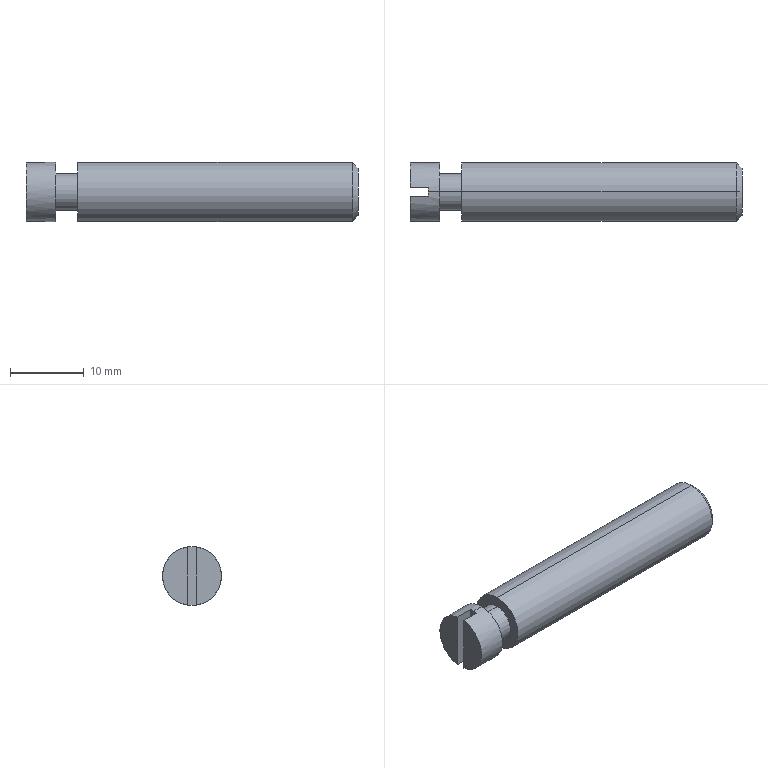Part | STEP file | 0217_Z_SBSPO8-45-1 | 1 solid | 16 faces | box 45 x 8 x 8 mm | volume 2139 mm3 | plane 8 | cylinder 6 | cone 2 | commonest cylinder face diameters 8 x4 5 x2
STEP:
#1=CARTESIAN_POINT('',(0.,0.,0.));
#2=DIRECTION('',(0.,0.,1.));
#3=DIRECTION('',(1.,0.,0.));
#4=AXIS2_PLACEMENT_3D('',#1,#2,#3);
#5=CARTESIAN_POINT('',(7.,0.,-4.));
#6=VERTEX_POINT('',#5);
#7=CARTESIAN_POINT('',(7.,0.,4.));
#8=VERTEX_POINT('',#7);
#9=CARTESIAN_POINT('',(7.,0.,0.));
#10=DIRECTION('',(1.,0.,0.));
#11=DIRECTION('',(0.,0.,-1.));
#12=AXIS2_PLACEMENT_3D('',#9,#10,#11);
#13=CIRCLE('',#12,4.);
#14=CARTESIAN_POINT('',(22.116,0.,0.));
#15=DIRECTION('',(1.,0.,0.));
#16=DIRECTION('',(0.,0.,-1.));
#17=AXIS2_PLACEMENT_3D('',#14,#15,#16);
#18=CYLINDRICAL_SURFACE('',#17,4.);
#19=CARTESIAN_POINT('',(0.,-15.117));
#20=DIRECTION('',(1.,0.));
#21=VECTOR('',#20,1.);
#22=LINE('',#19,#21);
#23=(GEOMETRIC_REPRESENTATION_CONTEXT(2)PARAMETRIC_REPRESENTATION_CONTEXT()REPRESENTATION_CONTEXT('',''));
#24=DEFINITIONAL_REPRESENTATION('',(#22),#23);
#25=PCURVE('',#18,#24);
#26=CARTESIAN_POINT('',(7.,4.,0.));
#27=DIRECTION('',(1.,0.,0.));
#28=DIRECTION('',(0.,0.,-1.));
#29=AXIS2_PLACEMENT_3D('',#26,#27,#28);
#30=PLANE('',#29);
#31=CARTESIAN_POINT('',(0.,-4.));
#32=DIRECTION('',(1.,0.));
#33=AXIS2_PLACEMENT_2D('',#31,#32);
#34=CIRCLE('',#33,4.);
#35=(GEOMETRIC_REPRESENTATION_CONTEXT(2)PARAMETRIC_REPRESENTATION_CONTEXT()REPRESENTATION_CONTEXT('',''));
#36=DEFINITIONAL_REPRESENTATION('',(#34),#35);
#37=PCURVE('',#30,#36);
#38=SURFACE_CURVE('',#13,(#25,#37),.PCURVE_S1.);
#39=EDGE_CURVE('',#6,#8,#38,.T.);
#40=ORIENTED_EDGE('',*,*,#39,.T.);
#41=CARTESIAN_POINT('',(44.233,0.,4.));
#42=VERTEX_POINT('',#41);
#43=CARTESIAN_POINT('',(22.116,0.,4.));
#44=DIRECTION('',(1.,0.,0.));
#45=VECTOR('',#44,1.);
#46=LINE('',#43,#45);
#47=CARTESIAN_POINT('',(3.142,0.));
#48=DIRECTION('',(0.,1.));
#49=VECTOR('',#48,1.);
#50=LINE('',#47,#49);
#51=(GEOMETRIC_REPRESENTATION_CONTEXT(2)PARAMETRIC_REPRESENTATION_CONTEXT()REPRESENTATION_CONTEXT('',''));
#52=DEFINITIONAL_REPRESENTATION('',(#50),#51);
#53=PCURVE('',#18,#52);
#54=CARTESIAN_POINT('',(22.116,0.,0.));
#55=DIRECTION('',(1.,0.,0.));
#56=DIRECTION('',(0.,0.,-1.));
#57=AXIS2_PLACEMENT_3D('',#54,#55,#56);
#58=CYLINDRICAL_SURFACE('',#57,4.);
#59=CARTESIAN_POINT('',(3.142,0.));
#60=DIRECTION('',(0.,1.));
#61=VECTOR('',#60,1.);
#62=LINE('',#59,#61);
#63=(GEOMETRIC_REPRESENTATION_CONTEXT(2)PARAMETRIC_REPRESENTATION_CONTEXT()REPRESENTATION_CONTEXT('',''));
#64=DEFINITIONAL_REPRESENTATION('',(#62),#63);
#65=PCURVE('',#58,#64);
#66=SURFACE_CURVE('',#46,(#53,#65),.PCURVE_S1.);
#67=EDGE_CURVE('',#8,#42,#66,.T.);
#68=ORIENTED_EDGE('',*,*,#67,.T.);
#69=CARTESIAN_POINT('',(44.233,0.,-4.));
#70=VERTEX_POINT('',#69);
#71=CARTESIAN_POINT('',(44.233,0.,0.));
#72=DIRECTION('',(-1.,0.,0.));
#73=DIRECTION('',(0.,0.,-1.));
#74=AXIS2_PLACEMENT_3D('',#71,#72,#73);
#75=CIRCLE('',#74,4.);
#76=CARTESIAN_POINT('',(6.283,22.116));
#77=DIRECTION('',(-1.,0.));
#78=VECTOR('',#77,1.);
#79=LINE('',#76,#78);
#80=(GEOMETRIC_REPRESENTATION_CONTEXT(2)PARAMETRIC_REPRESENTATION_CONTEXT()REPRESENTATION_CONTEXT('',''));
#81=DEFINITIONAL_REPRESENTATION('',(#79),#80);
#82=PCURVE('',#18,#81);
#83=CARTESIAN_POINT('',(44.233,0.,0.));
#84=DIRECTION('',(-1.,0.,0.));
#85=DIRECTION('',(0.,0.,1.));
#86=AXIS2_PLACEMENT_3D('',#83,#84,#85);
#87=CONICAL_SURFACE('',#86,4.,0.7854);
#88=CARTESIAN_POINT('',(-3.142,0.));
#89=DIRECTION('',(1.,0.));
#90=VECTOR('',#89,1.);
#91=LINE('',#88,#90);
#92=(GEOMETRIC_REPRESENTATION_CONTEXT(2)PARAMETRIC_REPRESENTATION_CONTEXT()REPRESENTATION_CONTEXT('',''));
#93=DEFINITIONAL_REPRESENTATION('',(#91),#92);
#94=PCURVE('',#87,#93);
#95=SURFACE_CURVE('',#75,(#82,#94),.PCURVE_S1.);
#96=EDGE_CURVE('',#42,#70,#95,.T.);
#97=ORIENTED_EDGE('',*,*,#96,.T.);
#98=CARTESIAN_POINT('',(22.116,0.,-4.));
#99=DIRECTION('',(1.,0.,0.));
#100=VECTOR('',#99,1.);
#101=LINE('',#98,#100);
#102=CARTESIAN_POINT('',(0.,0.));
#103=DIRECTION('',(0.,1.));
#104=VECTOR('',#103,1.);
#105=LINE('',#102,#104);
#106=(GEOMETRIC_REPRESENTATION_CONTEXT(2)PARAMETRIC_REPRESENTATION_CONTEXT()REPRESENTATION_CONTEXT('',''));
#107=DEFINITIONAL_REPRESENTATION('',(#105),#106);
#108=PCURVE('',#18,#107);
#109=CARTESIAN_POINT('',(6.283,0.));
#110=DIRECTION('',(0.,1.));
#111=VECTOR('',#110,1.);
#112=LINE('',#109,#111);
#113=(GEOMETRIC_REPRESENTATION_CONTEXT(2)PARAMETRIC_REPRESENTATION_CONTEXT()REPRESENTATION_CONTEXT('',''));
#114=DEFINITIONAL_REPRESENTATION('',(#112),#113);
#115=PCURVE('',#58,#114);
#116=SURFACE_CURVE('',#101,(#108,#115),.PCURVE_S1.);
#117=EDGE_CURVE('',#6,#70,#116,.T.);
#118=ORIENTED_EDGE('',*,*,#117,.F.);
#119=EDGE_LOOP('',(#40,#68,#97,#118));
#120=FACE_BOUND('',#119,.T.);
#121=ADVANCED_FACE('',(#120),#18,.T.);
#122=CARTESIAN_POINT('',(45.,0.,3.233));
#123=VERTEX_POINT('',#122);
#124=CARTESIAN_POINT('',(45.,0.,-3.233));
#125=VERTEX_POINT('',#124);
#126=CARTESIAN_POINT('',(45.,0.,0.));
#127=DIRECTION('',(-1.,0.,0.));
#128=DIRECTION('',(0.,0.,1.));
#129=AXIS2_PLACEMENT_3D('',#126,#127,#128);
#130=CIRCLE('',#129,3.233);
#131=CARTESIAN_POINT('',(0.,-0.767));
#132=DIRECTION('',(1.,0.));
#133=VECTOR('',#132,1.);
#134=LINE('',#131,#133);
#135=(GEOMETRIC_REPRESENTATION_CONTEXT(2)PARAMETRIC_REPRESENTATION_CONTEXT()REPRESENTATION_CONTEXT('',''));
#136=DEFINITIONAL_REPRESENTATION('',(#134),#135);
#137=PCURVE('',#87,#136);
#138=CARTESIAN_POINT('',(45.,1.617,0.));
#139=DIRECTION('',(1.,0.,0.));
#140=DIRECTION('',(0.,0.,-1.));
#141=AXIS2_PLACEMENT_3D('',#138,#139,#140);
#142=PLANE('',#141);
#143=CARTESIAN_POINT('',(-3.233,-1.617));
#144=CARTESIAN_POINT('',(-3.233,3.983));
#145=CARTESIAN_POINT('',(1.617,1.183));
#146=CARTESIAN_POINT('',(6.466,-1.617));
#147=CARTESIAN_POINT('',(1.617,-4.416));
#148=CARTESIAN_POINT('',(-3.233,-7.216));
#149=CARTESIAN_POINT('',(-3.233,-1.617));
#150=(BOUNDED_CURVE()B_SPLINE_CURVE(2,(#143,#144,#145,#146,#147,#148,#149),.UNSPECIFIED.,.T.,.F.)B_SPLINE_CURVE_WITH_KNOTS((1,2,2,2,2,1),(-2.094,0.,2.094,4.189,6.283,8.378),.UNSPECIFIED.)CURVE()GEOMETRIC_REPRESENTATION_ITEM()RATIONAL_B_SPLINE_CURVE((1.,0.5,1.,0.5,1.,0.5,1.))REPRESENTATION_ITEM(''));
#151=(GEOMETRIC_REPRESENTATION_CONTEXT(2)PARAMETRIC_REPRESENTATION_CONTEXT()REPRESENTATION_CONTEXT('',''));
#152=DEFINITIONAL_REPRESENTATION('',(#150),#151);
#153=PCURVE('',#142,#152);
#154=SURFACE_CURVE('',#130,(#137,#153),.PCURVE_S1.);
#155=EDGE_CURVE('',#123,#125,#154,.T.);
#156=ORIENTED_EDGE('',*,*,#155,.T.);
#157=CARTESIAN_POINT('',(44.233,0.,-4.));
#158=DIRECTION('',(-0.7071,0.,-0.7071));
#159=VECTOR('',#158,1.);
#160=LINE('',#157,#159);
#161=CARTESIAN_POINT('',(3.142,0.));
#162=DIRECTION('',(0.,1.));
#163=VECTOR('',#162,1.);
#164=LINE('',#161,#163);
#165=(GEOMETRIC_REPRESENTATION_CONTEXT(2)PARAMETRIC_REPRESENTATION_CONTEXT()REPRESENTATION_CONTEXT('',''));
#166=DEFINITIONAL_REPRESENTATION('',(#164),#165);
#167=PCURVE('',#87,#166);
#168=CARTESIAN_POINT('',(44.233,0.,0.));
#169=DIRECTION('',(-1.,0.,0.));
#170=DIRECTION('',(0.,0.,1.));
#171=AXIS2_PLACEMENT_3D('',#168,#169,#170);
#172=CONICAL_SURFACE('',#171,4.,0.7854);
#173=CARTESIAN_POINT('',(3.142,0.));
#174=DIRECTION('',(0.,1.));
#175=VECTOR('',#174,1.);
#176=LINE('',#173,#175);
#177=(GEOMETRIC_REPRESENTATION_CONTEXT(2)PARAMETRIC_REPRESENTATION_CONTEXT()REPRESENTATION_CONTEXT('',''));
#178=DEFINITIONAL_REPRESENTATION('',(#176),#177);
#179=PCURVE('',#172,#178);
#180=SURFACE_CURVE('',#160,(#167,#179),.PCURVE_S1.);
#181=EDGE_CURVE('',#125,#70,#180,.T.);
#182=ORIENTED_EDGE('',*,*,#181,.T.);
#183=ORIENTED_EDGE('',*,*,#96,.F.);
#184=CARTESIAN_POINT('',(44.233,0.,4.));
#185=DIRECTION('',(-0.7071,0.,0.7071));
#186=VECTOR('',#185,1.);
#187=LINE('',#184,#186);
#188=CARTESIAN_POINT('',(0.,0.));
#189=DIRECTION('',(0.,1.));
#190=VECTOR('',#189,1.);
#191=LINE('',#188,#190);
#192=(GEOMETRIC_REPRESENTATION_CONTEXT(2)PARAMETRIC_REPRESENTATION_CONTEXT()REPRESENTATION_CONTEXT('',''));
#193=DEFINITIONAL_REPRESENTATION('',(#191),#192);
#194=PCURVE('',#87,#193);
#195=CARTESIAN_POINT('',(6.283,0.));
#196=DIRECTION('',(0.,1.));
#197=VECTOR('',#196,1.);
#198=LINE('',#195,#197);
#199=(GEOMETRIC_REPRESENTATION_CONTEXT(2)PARAMETRIC_REPRESENTATION_CONTEXT()REPRESENTATION_CONTEXT('',''));
#200=DEFINITIONAL_REPRESENTATION('',(#198),#199);
#201=PCURVE('',#172,#200);
#202=SURFACE_CURVE('',#187,(#194,#201),.PCURVE_S1.);
#203=EDGE_CURVE('',#123,#42,#202,.T.);
#204=ORIENTED_EDGE('',*,*,#203,.F.);
#205=EDGE_LOOP('',(#156,#182,#183,#204));
#206=FACE_BOUND('',#205,.T.);
#207=ADVANCED_FACE('',(#206),#87,.T.);
#208=CARTESIAN_POINT('',(4.,0.,-2.5));
#209=VERTEX_POINT('',#208);
#210=CARTESIAN_POINT('',(4.,0.,2.5));
#211=VERTEX_POINT('',#210);
#212=CARTESIAN_POINT('',(4.,0.,0.));
#213=DIRECTION('',(1.,0.,0.));
#214=DIRECTION('',(0.,0.,-1.));
#215=AXIS2_PLACEMENT_3D('',#212,#213,#214);
#216=CIRCLE('',#215,2.5);
#217=CARTESIAN_POINT('',(5.5,0.,0.));
#218=DIRECTION('',(1.,0.,0.));
#219=DIRECTION('',(0.,0.,-1.));
#220=AXIS2_PLACEMENT_3D('',#217,#218,#219);
#221=CYLINDRICAL_SURFACE('',#220,2.5);
#222=CARTESIAN_POINT('',(0.,-1.5));
#223=DIRECTION('',(1.,0.));
#224=VECTOR('',#223,1.);
#225=LINE('',#222,#224);
#226=(GEOMETRIC_REPRESENTATION_CONTEXT(2)PARAMETRIC_REPRESENTATION_CONTEXT()REPRESENTATION_CONTEXT('',''));
#227=DEFINITIONAL_REPRESENTATION('',(#225),#226);
#228=PCURVE('',#221,#227);
#229=CARTESIAN_POINT('',(4.,4.,0.));
#230=DIRECTION('',(-1.,0.,0.));
#231=DIRECTION('',(0.,0.,1.));
#232=AXIS2_PLACEMENT_3D('',#229,#230,#231);
#233=PLANE('',#232);
#234=CARTESIAN_POINT('',(-2.5,-4.));
#235=CARTESIAN_POINT('',(-2.5,0.3301));
#236=CARTESIAN_POINT('',(1.25,-1.835));
#237=CARTESIAN_POINT('',(5.,-4.));
#238=CARTESIAN_POINT('',(1.25,-6.165));
#239=CARTESIAN_POINT('',(-2.5,-8.33));
#240=CARTESIAN_POINT('',(-2.5,-4.));
#241=(BOUNDED_CURVE()B_SPLINE_CURVE(2,(#234,#235,#236,#237,#238,#239,#240),.UNSPECIFIED.,.T.,.F.)B_SPLINE_CURVE_WITH_KNOTS((1,2,2,2,2,1),(-2.094,0.,2.094,4.189,6.283,8.378),.UNSPECIFIED.)CURVE()GEOMETRIC_REPRESENTATION_ITEM()RATIONAL_B_SPLINE_CURVE((1.,0.5,1.,0.5,1.,0.5,1.))REPRESENTATION_ITEM(''));
#242=(GEOMETRIC_REPRESENTATION_CONTEXT(2)PARAMETRIC_REPRESENTATION_CONTEXT()REPRESENTATION_CONTEXT('',''));
#243=DEFINITIONAL_REPRESENTATION('',(#241),#242);
#244=PCURVE('',#233,#243);
#245=SURFACE_CURVE('',#216,(#228,#244),.PCURVE_S1.);
#246=EDGE_CURVE('',#209,#211,#245,.T.);
#247=ORIENTED_EDGE('',*,*,#246,.T.);
#248=CARTESIAN_POINT('',(7.,0.,2.5));
#249=VERTEX_POINT('',#248);
#250=CARTESIAN_POINT('',(5.5,0.,2.5));
#251=DIRECTION('',(1.,0.,0.));
#252=VECTOR('',#251,1.);
#253=LINE('',#250,#252);
#254=CARTESIAN_POINT('',(3.142,0.));
#255=DIRECTION('',(0.,1.));
#256=VECTOR('',#255,1.);
#257=LINE('',#254,#256);
#258=(GEOMETRIC_REPRESENTATION_CONTEXT(2)PARAMETRIC_REPRESENTATION_CONTEXT()REPRESENTATION_CONTEXT('',''));
#259=DEFINITIONAL_REPRESENTATION('',(#257),#258);
#260=PCURVE('',#221,#259);
#261=CARTESIAN_POINT('',(5.5,0.,0.));
#262=DIRECTION('',(1.,0.,0.));
#263=DIRECTION('',(0.,0.,-1.));
#264=AXIS2_PLACEMENT_3D('',#261,#262,#263);
#265=CYLINDRICAL_SURFACE('',#264,2.5);
#266=CARTESIAN_POINT('',(3.142,0.));
#267=DIRECTION('',(0.,1.));
#268=VECTOR('',#267,1.);
#269=LINE('',#266,#268);
#270=(GEOMETRIC_REPRESENTATION_CONTEXT(2)PARAMETRIC_REPRESENTATION_CONTEXT()REPRESENTATION_CONTEXT('',''));
#271=DEFINITIONAL_REPRESENTATION('',(#269),#270);
#272=PCURVE('',#265,#271);
#273=SURFACE_CURVE('',#253,(#260,#272),.PCURVE_S1.);
#274=EDGE_CURVE('',#211,#249,#273,.T.);
#275=ORIENTED_EDGE('',*,*,#274,.T.);
#276=CARTESIAN_POINT('',(7.,0.,-2.5));
#277=VERTEX_POINT('',#276);
#278=CARTESIAN_POINT('',(7.,0.,0.));
#279=DIRECTION('',(-1.,0.,0.));
#280=DIRECTION('',(0.,0.,-1.));
#281=AXIS2_PLACEMENT_3D('',#278,#279,#280);
#282=CIRCLE('',#281,2.5);
#283=CARTESIAN_POINT('',(6.283,1.5));
#284=DIRECTION('',(-1.,0.));
#285=VECTOR('',#284,1.);
#286=LINE('',#283,#285);
#287=(GEOMETRIC_REPRESENTATION_CONTEXT(2)PARAMETRIC_REPRESENTATION_CONTEXT()REPRESENTATION_CONTEXT('',''));
#288=DEFINITIONAL_REPRESENTATION('',(#286),#287);
#289=PCURVE('',#221,#288);
#290=CARTESIAN_POINT('',(2.5,-4.));
#291=CARTESIAN_POINT('',(2.5,-8.33));
#292=CARTESIAN_POINT('',(-1.25,-6.165));
#293=CARTESIAN_POINT('',(-5.,-4.));
#294=CARTESIAN_POINT('',(-1.25,-1.835));
#295=CARTESIAN_POINT('',(2.5,0.3301));
#296=CARTESIAN_POINT('',(2.5,-4.));
#297=(BOUNDED_CURVE()B_SPLINE_CURVE(2,(#290,#291,#292,#293,#294,#295,#296),.UNSPECIFIED.,.T.,.F.)B_SPLINE_CURVE_WITH_KNOTS((1,2,2,2,2,1),(-2.094,0.,2.094,4.189,6.283,8.378),.UNSPECIFIED.)CURVE()GEOMETRIC_REPRESENTATION_ITEM()RATIONAL_B_SPLINE_CURVE((1.,0.5,1.,0.5,1.,0.5,1.))REPRESENTATION_ITEM(''));
#298=(GEOMETRIC_REPRESENTATION_CONTEXT(2)PARAMETRIC_REPRESENTATION_CONTEXT()REPRESENTATION_CONTEXT('',''));
#299=DEFINITIONAL_REPRESENTATION('',(#297),#298);
#300=PCURVE('',#30,#299);
#301=SURFACE_CURVE('',#282,(#289,#300),.PCURVE_S1.);
#302=EDGE_CURVE('',#249,#277,#301,.T.);
#303=ORIENTED_EDGE('',*,*,#302,.T.);
#304=CARTESIAN_POINT('',(5.5,0.,-2.5));
#305=DIRECTION('',(1.,0.,0.));
#306=VECTOR('',#305,1.);
#307=LINE('',#304,#306);
#308=CARTESIAN_POINT('',(0.,0.));
#309=DIRECTION('',(0.,1.));
#310=VECTOR('',#309,1.);
#311=LINE('',#308,#310);
#312=(GEOMETRIC_REPRESENTATION_CONTEXT(2)PARAMETRIC_REPRESENTATION_CONTEXT()REPRESENTATION_CONTEXT('',''));
#313=DEFINITIONAL_REPRESENTATION('',(#311),#312);
#314=PCURVE('',#221,#313);
#315=CARTESIAN_POINT('',(6.283,0.));
#316=DIRECTION('',(0.,1.));
#317=VECTOR('',#316,1.);
#318=LINE('',#315,#317);
#319=(GEOMETRIC_REPRESENTATION_CONTEXT(2)PARAMETRIC_REPRESENTATION_CONTEXT()REPRESENTATION_CONTEXT('',''));
#320=DEFINITIONAL_REPRESENTATION('',(#318),#319);
#321=PCURVE('',#265,#320);
#322=SURFACE_CURVE('',#307,(#314,#321),.PCURVE_S1.);
#323=EDGE_CURVE('',#209,#277,#322,.T.);
#324=ORIENTED_EDGE('',*,*,#323,.F.);
#325=EDGE_LOOP('',(#247,#275,#303,#324));
#326=FACE_BOUND('',#325,.T.);
#327=ADVANCED_FACE('',(#326),#221,.T.);
#328=CARTESIAN_POINT('',(2.5,0.6,3.955));
#329=VERTEX_POINT('',#328);
#330=CARTESIAN_POINT('',(2.5,0.,4.));
#331=VERTEX_POINT('',#330);
#332=CARTESIAN_POINT('',(2.5,0.,0.));
#333=DIRECTION('',(1.,0.,0.));
#334=DIRECTION('',(0.,0.,-1.));
#335=AXIS2_PLACEMENT_3D('',#332,#333,#334);
#336=CIRCLE('',#335,4.);
#337=CARTESIAN_POINT('',(22.116,0.,0.));
#338=DIRECTION('',(1.,0.,0.));
#339=DIRECTION('',(0.,0.,-1.));
#340=AXIS2_PLACEMENT_3D('',#337,#338,#339);
#341=CYLINDRICAL_SURFACE('',#340,4.);
#342=CARTESIAN_POINT('',(0.,-19.616));
#343=DIRECTION('',(1.,0.));
#344=VECTOR('',#343,1.);
#345=LINE('',#342,#344);
#346=(GEOMETRIC_REPRESENTATION_CONTEXT(2)PARAMETRIC_REPRESENTATION_CONTEXT()REPRESENTATION_CONTEXT('',''));
#347=DEFINITIONAL_REPRESENTATION('',(#345),#346);
#348=PCURVE('',#341,#347);
#349=CARTESIAN_POINT('',(2.5,-0.6,4.));
#350=DIRECTION('',(1.,0.,0.));
#351=DIRECTION('',(0.,0.,-1.));
#352=AXIS2_PLACEMENT_3D('',#349,#350,#351);
#353=PLANE('',#352);
#354=CARTESIAN_POINT('',(4.,0.6));
#355=DIRECTION('',(1.,0.));
#356=AXIS2_PLACEMENT_2D('',#354,#355);
#357=CIRCLE('',#356,4.);
#358=(GEOMETRIC_REPRESENTATION_CONTEXT(2)PARAMETRIC_REPRESENTATION_CONTEXT()REPRESENTATION_CONTEXT('',''));
#359=DEFINITIONAL_REPRESENTATION('',(#357),#358);
#360=PCURVE('',#353,#359);
#361=SURFACE_CURVE('',#336,(#348,#360),.PCURVE_S1.);
#362=EDGE_CURVE('',#329,#331,#361,.T.);
#363=ORIENTED_EDGE('',*,*,#362,.T.);
#364=CARTESIAN_POINT('',(4.,0.,4.));
#365=VERTEX_POINT('',#364);
#366=CARTESIAN_POINT('',(22.116,0.,4.));
#367=DIRECTION('',(1.,0.,0.));
#368=VECTOR('',#367,1.);
#369=LINE('',#366,#368);
#370=CARTESIAN_POINT('',(3.142,0.));
#371=DIRECTION('',(0.,1.));
#372=VECTOR('',#371,1.);
#373=LINE('',#370,#372);
#374=(GEOMETRIC_REPRESENTATION_CONTEXT(2)PARAMETRIC_REPRESENTATION_CONTEXT()REPRESENTATION_CONTEXT('',''));
#375=DEFINITIONAL_REPRESENTATION('',(#373),#374);
#376=PCURVE('',#341,#375);
#377=CARTESIAN_POINT('',(22.116,0.,0.));
#378=DIRECTION('',(1.,0.,0.));
#379=DIRECTION('',(0.,0.,-1.));
#380=AXIS2_PLACEMENT_3D('',#377,#378,#379);
#381=CYLINDRICAL_SURFACE('',#380,4.);
#382=CARTESIAN_POINT('',(3.142,0.));
#383=DIRECTION('',(0.,1.));
#384=VECTOR('',#383,1.);
#385=LINE('',#382,#384);
#386=(GEOMETRIC_REPRESENTATION_CONTEXT(2)PARAMETRIC_REPRESENTATION_CONTEXT()REPRESENTATION_CONTEXT('',''));
#387=DEFINITIONAL_REPRESENTATION('',(#385),#386);
#388=PCURVE('',#381,#387);
#389=SURFACE_CURVE('',#369,(#376,#388),.PCURVE_S1.);
#390=EDGE_CURVE('',#331,#365,#389,.T.);
#391=ORIENTED_EDGE('',*,*,#390,.T.);
#392=CARTESIAN_POINT('',(4.,0.,-4.));
#393=VERTEX_POINT('',#392);
#394=CARTESIAN_POINT('',(4.,0.,0.));
#395=DIRECTION('',(-1.,0.,0.));
#396=DIRECTION('',(0.,0.,-1.));
#397=AXIS2_PLACEMENT_3D('',#394,#395,#396);
#398=CIRCLE('',#397,4.);
#399=CARTESIAN_POINT('',(6.283,-18.116));
#400=DIRECTION('',(-1.,0.));
#401=VECTOR('',#400,1.);
#402=LINE('',#399,#401);
#403=(GEOMETRIC_REPRESENTATION_CONTEXT(2)PARAMETRIC_REPRESENTATION_CONTEXT()REPRESENTATION_CONTEXT('',''));
#404=DEFINITIONAL_REPRESENTATION('',(#402),#403);
#405=PCURVE('',#341,#404);
#406=CARTESIAN_POINT('',(0.,-4.));
#407=DIRECTION('',(-1.,0.));
#408=AXIS2_PLACEMENT_2D('',#406,#407);
#409=CIRCLE('',#408,4.);
#410=(GEOMETRIC_REPRESENTATION_CONTEXT(2)PARAMETRIC_REPRESENTATION_CONTEXT()REPRESENTATION_CONTEXT('',''));
#411=DEFINITIONAL_REPRESENTATION('',(#409),#410);
#412=PCURVE('',#233,#411);
#413=SURFACE_CURVE('',#398,(#405,#412),.PCURVE_S1.);
#414=EDGE_CURVE('',#365,#393,#413,.T.);
#415=ORIENTED_EDGE('',*,*,#414,.T.);
#416=CARTESIAN_POINT('',(2.5,0.,-4.));
#417=VERTEX_POINT('',#416);
#418=CARTESIAN_POINT('',(22.116,0.,-4.));
#419=DIRECTION('',(1.,0.,0.));
#420=VECTOR('',#419,1.);
#421=LINE('',#418,#420);
#422=CARTESIAN_POINT('',(0.,0.));
#423=DIRECTION('',(0.,1.));
#424=VECTOR('',#423,1.);
#425=LINE('',#422,#424);
#426=(GEOMETRIC_REPRESENTATION_CONTEXT(2)PARAMETRIC_REPRESENTATION_CONTEXT()REPRESENTATION_CONTEXT('',''));
#427=DEFINITIONAL_REPRESENTATION('',(#425),#426);
#428=PCURVE('',#341,#427);
#429=CARTESIAN_POINT('',(6.283,0.));
#430=DIRECTION('',(0.,1.));
#431=VECTOR('',#430,1.);
#432=LINE('',#429,#431);
#433=(GEOMETRIC_REPRESENTATION_CONTEXT(2)PARAMETRIC_REPRESENTATION_CONTEXT()REPRESENTATION_CONTEXT('',''));
#434=DEFINITIONAL_REPRESENTATION('',(#432),#433);
#435=PCURVE('',#381,#434);
#436=SURFACE_CURVE('',#421,(#428,#435),.PCURVE_S1.);
#437=EDGE_CURVE('',#417,#393,#436,.T.);
#438=ORIENTED_EDGE('',*,*,#437,.F.);
#439=CARTESIAN_POINT('',(2.5,0.6,-3.955));
#440=VERTEX_POINT('',#439);
#441=CARTESIAN_POINT('',(2.5,0.,0.));
#442=DIRECTION('',(1.,0.,0.));
#443=DIRECTION('',(0.,0.,-1.));
#444=AXIS2_PLACEMENT_3D('',#441,#442,#443);
#445=CIRCLE('',#444,4.);
#446=CARTESIAN_POINT('',(0.,-19.616));
#447=DIRECTION('',(1.,0.));
#448=VECTOR('',#447,1.);
#449=LINE('',#446,#448);
#450=(GEOMETRIC_REPRESENTATION_CONTEXT(2)PARAMETRIC_REPRESENTATION_CONTEXT()REPRESENTATION_CONTEXT('',''));
#451=DEFINITIONAL_REPRESENTATION('',(#449),#450);
#452=PCURVE('',#341,#451);
#453=CARTESIAN_POINT('',(4.,0.6));
#454=DIRECTION('',(1.,0.));
#455=AXIS2_PLACEMENT_2D('',#453,#454);
#456=CIRCLE('',#455,4.);
#457=(GEOMETRIC_REPRESENTATION_CONTEXT(2)PARAMETRIC_REPRESENTATION_CONTEXT()REPRESENTATION_CONTEXT('',''));
#458=DEFINITIONAL_REPRESENTATION('',(#456),#457);
#459=PCURVE('',#353,#458);
#460=SURFACE_CURVE('',#445,(#452,#459),.PCURVE_S1.);
#461=EDGE_CURVE('',#417,#440,#460,.T.);
#462=ORIENTED_EDGE('',*,*,#461,.T.);
#463=CARTESIAN_POINT('',(0.,0.6,-3.955));
#464=VERTEX_POINT('',#463);
#465=CARTESIAN_POINT('',(22.116,0.6,-3.955));
#466=DIRECTION('',(-1.,0.,0.));
#467=VECTOR('',#466,1.);
#468=LINE('',#465,#467);
#469=CARTESIAN_POINT('',(0.1506,0.));
#470=DIRECTION('',(0.,-1.));
#471=VECTOR('',#470,1.);
#472=LINE('',#469,#471);
#473=(GEOMETRIC_REPRESENTATION_CONTEXT(2)PARAMETRIC_REPRESENTATION_CONTEXT()REPRESENTATION_CONTEXT('',''));
#474=DEFINITIONAL_REPRESENTATION('',(#472),#473);
#475=PCURVE('',#341,#474);
#476=CARTESIAN_POINT('',(2.5,0.6,4.));
#477=DIRECTION('',(0.,1.,0.));
#478=DIRECTION('',(0.,0.,1.));
#479=AXIS2_PLACEMENT_3D('',#476,#477,#478);
#480=PLANE('',#479);
#481=CARTESIAN_POINT('',(-7.955,19.616));
#482=DIRECTION('',(0.,-1.));
#483=VECTOR('',#482,1.);
#484=LINE('',#481,#483);
#485=(GEOMETRIC_REPRESENTATION_CONTEXT(2)PARAMETRIC_REPRESENTATION_CONTEXT()REPRESENTATION_CONTEXT('',''));
#486=DEFINITIONAL_REPRESENTATION('',(#484),#485);
#487=PCURVE('',#480,#486);
#488=SURFACE_CURVE('',#468,(#475,#487),.PCURVE_S1.);
#489=EDGE_CURVE('',#440,#464,#488,.T.);
#490=ORIENTED_EDGE('',*,*,#489,.T.);
#491=CARTESIAN_POINT('',(0.,0.6,3.955));
#492=VERTEX_POINT('',#491);
#493=CARTESIAN_POINT('',(0.,0.,0.));
#494=DIRECTION('',(1.,0.,0.));
#495=DIRECTION('',(0.,0.,-1.));
#496=AXIS2_PLACEMENT_3D('',#493,#494,#495);
#497=CIRCLE('',#496,4.);
#498=CARTESIAN_POINT('',(0.,-22.116));
#499=DIRECTION('',(1.,0.));
#500=VECTOR('',#499,1.);
#501=LINE('',#498,#500);
#502=(GEOMETRIC_REPRESENTATION_CONTEXT(2)PARAMETRIC_REPRESENTATION_CONTEXT()REPRESENTATION_CONTEXT('',''));
#503=DEFINITIONAL_REPRESENTATION('',(#501),#502);
#504=PCURVE('',#341,#503);
#505=CARTESIAN_POINT('',(0.,2.,0.));
#506=DIRECTION('',(-1.,0.,0.));
#507=DIRECTION('',(0.,0.,1.));
#508=AXIS2_PLACEMENT_3D('',#505,#506,#507);
#509=PLANE('',#508);
#510=CARTESIAN_POINT('',(-4.,-2.));
#511=CARTESIAN_POINT('',(-4.,4.928));
#512=CARTESIAN_POINT('',(2.,1.464));
#513=CARTESIAN_POINT('',(8.,-2.));
#514=CARTESIAN_POINT('',(2.,-5.464));
#515=CARTESIAN_POINT('',(-4.,-8.928));
#516=CARTESIAN_POINT('',(-4.,-2.));
#517=(BOUNDED_CURVE()B_SPLINE_CURVE(2,(#510,#511,#512,#513,#514,#515,#516),.UNSPECIFIED.,.T.,.F.)B_SPLINE_CURVE_WITH_KNOTS((1,2,2,2,2,1),(-2.094,0.,2.094,4.189,6.283,8.378),.UNSPECIFIED.)CURVE()GEOMETRIC_REPRESENTATION_ITEM()RATIONAL_B_SPLINE_CURVE((1.,0.5,1.,0.5,1.,0.5,1.))REPRESENTATION_ITEM(''));
#518=(GEOMETRIC_REPRESENTATION_CONTEXT(2)PARAMETRIC_REPRESENTATION_CONTEXT()REPRESENTATION_CONTEXT('',''));
#519=DEFINITIONAL_REPRESENTATION('',(#517),#518);
#520=PCURVE('',#509,#519);
#521=SURFACE_CURVE('',#497,(#504,#520),.PCURVE_S1.);
#522=EDGE_CURVE('',#464,#492,#521,.T.);
#523=ORIENTED_EDGE('',*,*,#522,.T.);
#524=CARTESIAN_POINT('',(22.116,0.6,3.955));
#525=DIRECTION('',(1.,0.,0.));
#526=VECTOR('',#525,1.);
#527=LINE('',#524,#526);
#528=CARTESIAN_POINT('',(2.991,0.));
#529=DIRECTION('',(0.,1.));
#530=VECTOR('',#529,1.);
#531=LINE('',#528,#530);
#532=(GEOMETRIC_REPRESENTATION_CONTEXT(2)PARAMETRIC_REPRESENTATION_CONTEXT()REPRESENTATION_CONTEXT('',''));
#533=DEFINITIONAL_REPRESENTATION('',(#531),#532);
#534=PCURVE('',#341,#533);
#535=CARTESIAN_POINT('',(-0.04526,19.616));
#536=DIRECTION('',(0.,1.));
#537=VECTOR('',#536,1.);
#538=LINE('',#535,#537);
#539=(GEOMETRIC_REPRESENTATION_CONTEXT(2)PARAMETRIC_REPRESENTATION_CONTEXT()REPRESENTATION_CONTEXT('',''));
#540=DEFINITIONAL_REPRESENTATION('',(#538),#539);
#541=PCURVE('',#480,#540);
#542=SURFACE_CURVE('',#527,(#534,#541),.PCURVE_S1.);
#543=EDGE_CURVE('',#492,#329,#542,.T.);
#544=ORIENTED_EDGE('',*,*,#543,.T.);
#545=EDGE_LOOP('',(#363,#391,#415,#438,#462,#490,#523,#544));
#546=FACE_BOUND('',#545,.T.);
#547=ADVANCED_FACE('',(#546),#341,.T.);
#548=ORIENTED_EDGE('',*,*,#67,.F.);
#549=CARTESIAN_POINT('',(7.,0.,0.));
#550=DIRECTION('',(1.,0.,0.));
#551=DIRECTION('',(0.,0.,-1.));
#552=AXIS2_PLACEMENT_3D('',#549,#550,#551);
#553=CIRCLE('',#552,4.);
#554=CARTESIAN_POINT('',(0.,-15.117));
#555=DIRECTION('',(1.,0.));
#556=VECTOR('',#555,1.);
#557=LINE('',#554,#556);
#558=(GEOMETRIC_REPRESENTATION_CONTEXT(2)PARAMETRIC_REPRESENTATION_CONTEXT()REPRESENTATION_CONTEXT('',''));
#559=DEFINITIONAL_REPRESENTATION('',(#557),#558);
#560=PCURVE('',#58,#559);
#561=CARTESIAN_POINT('',(0.,-4.));
#562=DIRECTION('',(1.,0.));
#563=AXIS2_PLACEMENT_2D('',#561,#562);
#564=CIRCLE('',#563,4.);
#565=(GEOMETRIC_REPRESENTATION_CONTEXT(2)PARAMETRIC_REPRESENTATION_CONTEXT()REPRESENTATION_CONTEXT('',''));
#566=DEFINITIONAL_REPRESENTATION('',(#564),#565);
#567=PCURVE('',#30,#566);
#568=SURFACE_CURVE('',#553,(#560,#567),.PCURVE_S1.);
#569=EDGE_CURVE('',#8,#6,#568,.T.);
#570=ORIENTED_EDGE('',*,*,#569,.T.);
#571=ORIENTED_EDGE('',*,*,#117,.T.);
#572=CARTESIAN_POINT('',(44.233,0.,0.));
#573=DIRECTION('',(-1.,0.,0.));
#574=DIRECTION('',(0.,0.,-1.));
#575=AXIS2_PLACEMENT_3D('',#572,#573,#574);
#576=CIRCLE('',#575,4.);
#577=CARTESIAN_POINT('',(6.283,22.116));
#578=DIRECTION('',(-1.,0.));
#579=VECTOR('',#578,1.);
#580=LINE('',#577,#579);
#581=(GEOMETRIC_REPRESENTATION_CONTEXT(2)PARAMETRIC_REPRESENTATION_CONTEXT()REPRESENTATION_CONTEXT('',''));
#582=DEFINITIONAL_REPRESENTATION('',(#580),#581);
#583=PCURVE('',#58,#582);
#584=CARTESIAN_POINT('',(3.142,0.));
#585=DIRECTION('',(1.,0.));
#586=VECTOR('',#585,1.);
#587=LINE('',#584,#586);
#588=(GEOMETRIC_REPRESENTATION_CONTEXT(2)PARAMETRIC_REPRESENTATION_CONTEXT()REPRESENTATION_CONTEXT('',''));
#589=DEFINITIONAL_REPRESENTATION('',(#587),#588);
#590=PCURVE('',#172,#589);
#591=SURFACE_CURVE('',#576,(#583,#590),.PCURVE_S1.);
#592=EDGE_CURVE('',#70,#42,#591,.T.);
#593=ORIENTED_EDGE('',*,*,#592,.T.);
#594=EDGE_LOOP('',(#548,#570,#571,#593));
#595=FACE_BOUND('',#594,.T.);
#596=ADVANCED_FACE('',(#595),#58,.T.);
#597=CARTESIAN_POINT('',(7.,0.,0.));
#598=DIRECTION('',(-1.,0.,0.));
#599=DIRECTION('',(0.,0.,-1.));
#600=AXIS2_PLACEMENT_3D('',#597,#598,#599);
#601=CIRCLE('',#600,2.5);
#602=CARTESIAN_POINT('',(2.5,-4.));
#603=CARTESIAN_POINT('',(2.5,-8.33));
#604=CARTESIAN_POINT('',(-1.25,-6.165));
#605=CARTESIAN_POINT('',(-5.,-4.));
#606=CARTESIAN_POINT('',(-1.25,-1.835));
#607=CARTESIAN_POINT('',(2.5,0.3301));
#608=CARTESIAN_POINT('',(2.5,-4.));
#609=(BOUNDED_CURVE()B_SPLINE_CURVE(2,(#602,#603,#604,#605,#606,#607,#608),.UNSPECIFIED.,.T.,.F.)B_SPLINE_CURVE_WITH_KNOTS((1,2,2,2,2,1),(-2.094,0.,2.094,4.189,6.283,8.378),.UNSPECIFIED.)CURVE()GEOMETRIC_REPRESENTATION_ITEM()RATIONAL_B_SPLINE_CURVE((1.,0.5,1.,0.5,1.,0.5,1.))REPRESENTATION_ITEM(''));
#610=(GEOMETRIC_REPRESENTATION_CONTEXT(2)PARAMETRIC_REPRESENTATION_CONTEXT()REPRESENTATION_CONTEXT('',''));
#611=DEFINITIONAL_REPRESENTATION('',(#609),#610);
#612=PCURVE('',#30,#611);
#613=CARTESIAN_POINT('',(6.283,1.5));
#614=DIRECTION('',(-1.,0.));
#615=VECTOR('',#614,1.);
#616=LINE('',#613,#615);
#617=(GEOMETRIC_REPRESENTATION_CONTEXT(2)PARAMETRIC_REPRESENTATION_CONTEXT()REPRESENTATION_CONTEXT('',''));
#618=DEFINITIONAL_REPRESENTATION('',(#616),#617);
#619=PCURVE('',#265,#618);
#620=SURFACE_CURVE('',#601,(#612,#619),.PCURVE_S1.);
#621=EDGE_CURVE('',#277,#249,#620,.T.);
#622=ORIENTED_EDGE('',*,*,#621,.F.);
#623=ORIENTED_EDGE('',*,*,#302,.F.);
#624=EDGE_LOOP('',(#622,#623));
#625=FACE_BOUND('',#624,.T.);
#626=ORIENTED_EDGE('',*,*,#39,.F.);
#627=ORIENTED_EDGE('',*,*,#569,.F.);
#628=EDGE_LOOP('',(#626,#627));
#629=FACE_BOUND('',#628,.T.);
#630=ADVANCED_FACE('',(#625,#629),#30,.F.);
#631=ORIENTED_EDGE('',*,*,#181,.F.);
#632=CARTESIAN_POINT('',(45.,0.,0.));
#633=DIRECTION('',(-1.,0.,0.));
#634=DIRECTION('',(0.,0.,1.));
#635=AXIS2_PLACEMENT_3D('',#632,#633,#634);
#636=CIRCLE('',#635,3.233);
#637=CARTESIAN_POINT('',(0.,-0.767));
#638=DIRECTION('',(1.,0.));
#639=VECTOR('',#638,1.);
#640=LINE('',#637,#639);
#641=(GEOMETRIC_REPRESENTATION_CONTEXT(2)PARAMETRIC_REPRESENTATION_CONTEXT()REPRESENTATION_CONTEXT('',''));
#642=DEFINITIONAL_REPRESENTATION('',(#640),#641);
#643=PCURVE('',#172,#642);
#644=CARTESIAN_POINT('',(-3.233,-1.617));
#645=CARTESIAN_POINT('',(-3.233,3.983));
#646=CARTESIAN_POINT('',(1.617,1.183));
#647=CARTESIAN_POINT('',(6.466,-1.617));
#648=CARTESIAN_POINT('',(1.617,-4.416));
#649=CARTESIAN_POINT('',(-3.233,-7.216));
#650=CARTESIAN_POINT('',(-3.233,-1.617));
#651=(BOUNDED_CURVE()B_SPLINE_CURVE(2,(#644,#645,#646,#647,#648,#649,#650),.UNSPECIFIED.,.T.,.F.)B_SPLINE_CURVE_WITH_KNOTS((1,2,2,2,2,1),(-2.094,0.,2.094,4.189,6.283,8.378),.UNSPECIFIED.)CURVE()GEOMETRIC_REPRESENTATION_ITEM()RATIONAL_B_SPLINE_CURVE((1.,0.5,1.,0.5,1.,0.5,1.))REPRESENTATION_ITEM(''));
#652=(GEOMETRIC_REPRESENTATION_CONTEXT(2)PARAMETRIC_REPRESENTATION_CONTEXT()REPRESENTATION_CONTEXT('',''));
#653=DEFINITIONAL_REPRESENTATION('',(#651),#652);
#654=PCURVE('',#142,#653);
#655=SURFACE_CURVE('',#636,(#643,#654),.PCURVE_S1.);
#656=EDGE_CURVE('',#125,#123,#655,.T.);
#657=ORIENTED_EDGE('',*,*,#656,.T.);
#658=ORIENTED_EDGE('',*,*,#203,.T.);
#659=ORIENTED_EDGE('',*,*,#592,.F.);
#660=EDGE_LOOP('',(#631,#657,#658,#659));
#661=FACE_BOUND('',#660,.T.);
#662=ADVANCED_FACE('',(#661),#172,.T.);
#663=ORIENTED_EDGE('',*,*,#274,.F.);
#664=CARTESIAN_POINT('',(4.,0.,0.));
#665=DIRECTION('',(1.,0.,0.));
#666=DIRECTION('',(0.,0.,-1.));
#667=AXIS2_PLACEMENT_3D('',#664,#665,#666);
#668=CIRCLE('',#667,2.5);
#669=CARTESIAN_POINT('',(0.,-1.5));
#670=DIRECTION('',(1.,0.));
#671=VECTOR('',#670,1.);
#672=LINE('',#669,#671);
#673=(GEOMETRIC_REPRESENTATION_CONTEXT(2)PARAMETRIC_REPRESENTATION_CONTEXT()REPRESENTATION_CONTEXT('',''));
#674=DEFINITIONAL_REPRESENTATION('',(#672),#673);
#675=PCURVE('',#265,#674);
#676=CARTESIAN_POINT('',(-2.5,-4.));
#677=CARTESIAN_POINT('',(-2.5,0.3301));
#678=CARTESIAN_POINT('',(1.25,-1.835));
#679=CARTESIAN_POINT('',(5.,-4.));
#680=CARTESIAN_POINT('',(1.25,-6.165));
#681=CARTESIAN_POINT('',(-2.5,-8.33));
#682=CARTESIAN_POINT('',(-2.5,-4.));
#683=(BOUNDED_CURVE()B_SPLINE_CURVE(2,(#676,#677,#678,#679,#680,#681,#682),.UNSPECIFIED.,.T.,.F.)B_SPLINE_CURVE_WITH_KNOTS((1,2,2,2,2,1),(-2.094,0.,2.094,4.189,6.283,8.378),.UNSPECIFIED.)CURVE()GEOMETRIC_REPRESENTATION_ITEM()RATIONAL_B_SPLINE_CURVE((1.,0.5,1.,0.5,1.,0.5,1.))REPRESENTATION_ITEM(''));
#684=(GEOMETRIC_REPRESENTATION_CONTEXT(2)PARAMETRIC_REPRESENTATION_CONTEXT()REPRESENTATION_CONTEXT('',''));
#685=DEFINITIONAL_REPRESENTATION('',(#683),#684);
#686=PCURVE('',#233,#685);
#687=SURFACE_CURVE('',#668,(#675,#686),.PCURVE_S1.);
#688=EDGE_CURVE('',#211,#209,#687,.T.);
#689=ORIENTED_EDGE('',*,*,#688,.T.);
#690=ORIENTED_EDGE('',*,*,#323,.T.);
#691=ORIENTED_EDGE('',*,*,#621,.T.);
#692=EDGE_LOOP('',(#663,#689,#690,#691));
#693=FACE_BOUND('',#692,.T.);
#694=ADVANCED_FACE('',(#693),#265,.T.);
#695=ORIENTED_EDGE('',*,*,#155,.F.);
#696=ORIENTED_EDGE('',*,*,#656,.F.);
#697=EDGE_LOOP('',(#695,#696));
#698=FACE_BOUND('',#697,.T.);
#699=ADVANCED_FACE('',(#698),#142,.T.);
#700=ORIENTED_EDGE('',*,*,#246,.F.);
#701=ORIENTED_EDGE('',*,*,#688,.F.);
#702=EDGE_LOOP('',(#700,#701));
#703=FACE_BOUND('',#702,.T.);
#704=CARTESIAN_POINT('',(4.,0.,0.));
#705=DIRECTION('',(-1.,0.,0.));
#706=DIRECTION('',(0.,0.,-1.));
#707=AXIS2_PLACEMENT_3D('',#704,#705,#706);
#708=CIRCLE('',#707,4.);
#709=CARTESIAN_POINT('',(0.,-4.));
#710=DIRECTION('',(-1.,0.));
#711=AXIS2_PLACEMENT_2D('',#709,#710);
#712=CIRCLE('',#711,4.);
#713=(GEOMETRIC_REPRESENTATION_CONTEXT(2)PARAMETRIC_REPRESENTATION_CONTEXT()REPRESENTATION_CONTEXT('',''));
#714=DEFINITIONAL_REPRESENTATION('',(#712),#713);
#715=PCURVE('',#233,#714);
#716=CARTESIAN_POINT('',(6.283,-18.116));
#717=DIRECTION('',(-1.,0.));
#718=VECTOR('',#717,1.);
#719=LINE('',#716,#718);
#720=(GEOMETRIC_REPRESENTATION_CONTEXT(2)PARAMETRIC_REPRESENTATION_CONTEXT()REPRESENTATION_CONTEXT('',''));
#721=DEFINITIONAL_REPRESENTATION('',(#719),#720);
#722=PCURVE('',#381,#721);
#723=SURFACE_CURVE('',#708,(#715,#722),.PCURVE_S1.);
#724=EDGE_CURVE('',#393,#365,#723,.T.);
#725=ORIENTED_EDGE('',*,*,#724,.F.);
#726=ORIENTED_EDGE('',*,*,#414,.F.);
#727=EDGE_LOOP('',(#725,#726));
#728=FACE_BOUND('',#727,.T.);
#729=ADVANCED_FACE('',(#703,#728),#233,.F.);
#730=ORIENTED_EDGE('',*,*,#390,.F.);
#731=CARTESIAN_POINT('',(2.5,-0.6,3.955));
#732=VERTEX_POINT('',#731);
#733=CARTESIAN_POINT('',(2.5,0.,0.));
#734=DIRECTION('',(1.,0.,0.));
#735=DIRECTION('',(0.,0.,-1.));
#736=AXIS2_PLACEMENT_3D('',#733,#734,#735);
#737=CIRCLE('',#736,4.);
#738=CARTESIAN_POINT('',(0.,-19.616));
#739=DIRECTION('',(1.,0.));
#740=VECTOR('',#739,1.);
#741=LINE('',#738,#740);
#742=(GEOMETRIC_REPRESENTATION_CONTEXT(2)PARAMETRIC_REPRESENTATION_CONTEXT()REPRESENTATION_CONTEXT('',''));
#743=DEFINITIONAL_REPRESENTATION('',(#741),#742);
#744=PCURVE('',#381,#743);
#745=CARTESIAN_POINT('',(4.,0.6));
#746=DIRECTION('',(1.,0.));
#747=AXIS2_PLACEMENT_2D('',#745,#746);
#748=CIRCLE('',#747,4.);
#749=(GEOMETRIC_REPRESENTATION_CONTEXT(2)PARAMETRIC_REPRESENTATION_CONTEXT()REPRESENTATION_CONTEXT('',''));
#750=DEFINITIONAL_REPRESENTATION('',(#748),#749);
#751=PCURVE('',#353,#750);
#752=SURFACE_CURVE('',#737,(#744,#751),.PCURVE_S1.);
#753=EDGE_CURVE('',#331,#732,#752,.T.);
#754=ORIENTED_EDGE('',*,*,#753,.T.);
#755=CARTESIAN_POINT('',(0.,-0.6,3.955));
#756=VERTEX_POINT('',#755);
#757=CARTESIAN_POINT('',(22.116,-0.6,3.955));
#758=DIRECTION('',(-1.,0.,0.));
#759=VECTOR('',#758,1.);
#760=LINE('',#757,#759);
#761=CARTESIAN_POINT('',(3.292,0.));
#762=DIRECTION('',(0.,-1.));
#763=VECTOR('',#762,1.);
#764=LINE('',#761,#763);
#765=(GEOMETRIC_REPRESENTATION_CONTEXT(2)PARAMETRIC_REPRESENTATION_CONTEXT()REPRESENTATION_CONTEXT('',''));
#766=DEFINITIONAL_REPRESENTATION('',(#764),#765);
#767=PCURVE('',#381,#766);
#768=CARTESIAN_POINT('',(0.,-0.6,4.));
#769=DIRECTION('',(0.,-1.,0.));
#770=DIRECTION('',(0.,0.,-1.));
#771=AXIS2_PLACEMENT_3D('',#768,#769,#770);
#772=PLANE('',#771);
#773=CARTESIAN_POINT('',(0.04526,22.116));
#774=DIRECTION('',(0.,-1.));
#775=VECTOR('',#774,1.);
#776=LINE('',#773,#775);
#777=(GEOMETRIC_REPRESENTATION_CONTEXT(2)PARAMETRIC_REPRESENTATION_CONTEXT()REPRESENTATION_CONTEXT('',''));
#778=DEFINITIONAL_REPRESENTATION('',(#776),#777);
#779=PCURVE('',#772,#778);
#780=SURFACE_CURVE('',#760,(#767,#779),.PCURVE_S1.);
#781=EDGE_CURVE('',#732,#756,#780,.T.);
#782=ORIENTED_EDGE('',*,*,#781,.T.);
#783=CARTESIAN_POINT('',(0.,-0.6,-3.955));
#784=VERTEX_POINT('',#783);
#785=CARTESIAN_POINT('',(0.,0.,0.));
#786=DIRECTION('',(1.,0.,0.));
#787=DIRECTION('',(0.,0.,-1.));
#788=AXIS2_PLACEMENT_3D('',#785,#786,#787);
#789=CIRCLE('',#788,4.);
#790=CARTESIAN_POINT('',(0.,-22.116));
#791=DIRECTION('',(1.,0.));
#792=VECTOR('',#791,1.);
#793=LINE('',#790,#792);
#794=(GEOMETRIC_REPRESENTATION_CONTEXT(2)PARAMETRIC_REPRESENTATION_CONTEXT()REPRESENTATION_CONTEXT('',''));
#795=DEFINITIONAL_REPRESENTATION('',(#793),#794);
#796=PCURVE('',#381,#795);
#797=CARTESIAN_POINT('',(0.,2.,0.));
#798=DIRECTION('',(-1.,0.,0.));
#799=DIRECTION('',(0.,0.,1.));
#800=AXIS2_PLACEMENT_3D('',#797,#798,#799);
#801=PLANE('',#800);
#802=CARTESIAN_POINT('',(-4.,-2.));
#803=CARTESIAN_POINT('',(-4.,4.928));
#804=CARTESIAN_POINT('',(2.,1.464));
#805=CARTESIAN_POINT('',(8.,-2.));
#806=CARTESIAN_POINT('',(2.,-5.464));
#807=CARTESIAN_POINT('',(-4.,-8.928));
#808=CARTESIAN_POINT('',(-4.,-2.));
#809=(BOUNDED_CURVE()B_SPLINE_CURVE(2,(#802,#803,#804,#805,#806,#807,#808),.UNSPECIFIED.,.T.,.F.)B_SPLINE_CURVE_WITH_KNOTS((1,2,2,2,2,1),(-2.094,0.,2.094,4.189,6.283,8.378),.UNSPECIFIED.)CURVE()GEOMETRIC_REPRESENTATION_ITEM()RATIONAL_B_SPLINE_CURVE((1.,0.5,1.,0.5,1.,0.5,1.))REPRESENTATION_ITEM(''));
#810=(GEOMETRIC_REPRESENTATION_CONTEXT(2)PARAMETRIC_REPRESENTATION_CONTEXT()REPRESENTATION_CONTEXT('',''));
#811=DEFINITIONAL_REPRESENTATION('',(#809),#810);
#812=PCURVE('',#801,#811);
#813=SURFACE_CURVE('',#789,(#796,#812),.PCURVE_S1.);
#814=EDGE_CURVE('',#756,#784,#813,.T.);
#815=ORIENTED_EDGE('',*,*,#814,.T.);
#816=CARTESIAN_POINT('',(2.5,-0.6,-3.955));
#817=VERTEX_POINT('',#816);
#818=CARTESIAN_POINT('',(22.116,-0.6,-3.955));
#819=DIRECTION('',(1.,0.,0.));
#820=VECTOR('',#819,1.);
#821=LINE('',#818,#820);
#822=CARTESIAN_POINT('',(6.133,0.));
#823=DIRECTION('',(0.,1.));
#824=VECTOR('',#823,1.);
#825=LINE('',#822,#824);
#826=(GEOMETRIC_REPRESENTATION_CONTEXT(2)PARAMETRIC_REPRESENTATION_CONTEXT()REPRESENTATION_CONTEXT('',''));
#827=DEFINITIONAL_REPRESENTATION('',(#825),#826);
#828=PCURVE('',#381,#827);
#829=CARTESIAN_POINT('',(7.955,22.116));
#830=DIRECTION('',(0.,1.));
#831=VECTOR('',#830,1.);
#832=LINE('',#829,#831);
#833=(GEOMETRIC_REPRESENTATION_CONTEXT(2)PARAMETRIC_REPRESENTATION_CONTEXT()REPRESENTATION_CONTEXT('',''));
#834=DEFINITIONAL_REPRESENTATION('',(#832),#833);
#835=PCURVE('',#772,#834);
#836=SURFACE_CURVE('',#821,(#828,#835),.PCURVE_S1.);
#837=EDGE_CURVE('',#784,#817,#836,.T.);
#838=ORIENTED_EDGE('',*,*,#837,.T.);
#839=CARTESIAN_POINT('',(2.5,0.,0.));
#840=DIRECTION('',(1.,0.,0.));
#841=DIRECTION('',(0.,0.,-1.));
#842=AXIS2_PLACEMENT_3D('',#839,#840,#841);
#843=CIRCLE('',#842,4.);
#844=CARTESIAN_POINT('',(0.,-19.616));
#845=DIRECTION('',(1.,0.));
#846=VECTOR('',#845,1.);
#847=LINE('',#844,#846);
#848=(GEOMETRIC_REPRESENTATION_CONTEXT(2)PARAMETRIC_REPRESENTATION_CONTEXT()REPRESENTATION_CONTEXT('',''));
#849=DEFINITIONAL_REPRESENTATION('',(#847),#848);
#850=PCURVE('',#381,#849);
#851=CARTESIAN_POINT('',(4.,0.6));
#852=DIRECTION('',(1.,0.));
#853=AXIS2_PLACEMENT_2D('',#851,#852);
#854=CIRCLE('',#853,4.);
#855=(GEOMETRIC_REPRESENTATION_CONTEXT(2)PARAMETRIC_REPRESENTATION_CONTEXT()REPRESENTATION_CONTEXT('',''));
#856=DEFINITIONAL_REPRESENTATION('',(#854),#855);
#857=PCURVE('',#353,#856);
#858=SURFACE_CURVE('',#843,(#850,#857),.PCURVE_S1.);
#859=EDGE_CURVE('',#817,#417,#858,.T.);
#860=ORIENTED_EDGE('',*,*,#859,.T.);
#861=ORIENTED_EDGE('',*,*,#437,.T.);
#862=ORIENTED_EDGE('',*,*,#724,.T.);
#863=EDGE_LOOP('',(#730,#754,#782,#815,#838,#860,#861,#862));
#864=FACE_BOUND('',#863,.T.);
#865=ADVANCED_FACE('',(#864),#381,.T.);
#866=CARTESIAN_POINT('',(0.,-0.6,0.));
#867=DIRECTION('',(0.,0.,-1.));
#868=VECTOR('',#867,1.);
#869=LINE('',#866,#868);
#870=CARTESIAN_POINT('',(0.,-2.6));
#871=DIRECTION('',(-1.,0.));
#872=VECTOR('',#871,1.);
#873=LINE('',#870,#872);
#874=(GEOMETRIC_REPRESENTATION_CONTEXT(2)PARAMETRIC_REPRESENTATION_CONTEXT()REPRESENTATION_CONTEXT('',''));
#875=DEFINITIONAL_REPRESENTATION('',(#873),#874);
#876=PCURVE('',#801,#875);
#877=CARTESIAN_POINT('',(4.,0.));
#878=DIRECTION('',(1.,0.));
#879=VECTOR('',#878,1.);
#880=LINE('',#877,#879);
#881=(GEOMETRIC_REPRESENTATION_CONTEXT(2)PARAMETRIC_REPRESENTATION_CONTEXT()REPRESENTATION_CONTEXT('',''));
#882=DEFINITIONAL_REPRESENTATION('',(#880),#881);
#883=PCURVE('',#772,#882);
#884=SURFACE_CURVE('',#869,(#876,#883),.PCURVE_S1.);
#885=EDGE_CURVE('',#756,#784,#884,.T.);
#886=ORIENTED_EDGE('',*,*,#885,.T.);
#887=ORIENTED_EDGE('',*,*,#814,.F.);
#888=EDGE_LOOP('',(#886,#887));
#889=FACE_BOUND('',#888,.T.);
#890=ADVANCED_FACE('',(#889),#801,.T.);
#891=ORIENTED_EDGE('',*,*,#885,.F.);
#892=ORIENTED_EDGE('',*,*,#781,.F.);
#893=CARTESIAN_POINT('',(2.5,-0.6,4.));
#894=DIRECTION('',(0.,0.,1.));
#895=VECTOR('',#894,1.);
#896=LINE('',#893,#895);
#897=CARTESIAN_POINT('',(0.,2.5));
#898=DIRECTION('',(-1.,0.));
#899=VECTOR('',#898,1.);
#900=LINE('',#897,#899);
#901=(GEOMETRIC_REPRESENTATION_CONTEXT(2)PARAMETRIC_REPRESENTATION_CONTEXT()REPRESENTATION_CONTEXT('',''));
#902=DEFINITIONAL_REPRESENTATION('',(#900),#901);
#903=PCURVE('',#772,#902);
#904=CARTESIAN_POINT('',(0.,0.));
#905=DIRECTION('',(-1.,0.));
#906=VECTOR('',#905,1.);
#907=LINE('',#904,#906);
#908=(GEOMETRIC_REPRESENTATION_CONTEXT(2)PARAMETRIC_REPRESENTATION_CONTEXT()REPRESENTATION_CONTEXT('',''));
#909=DEFINITIONAL_REPRESENTATION('',(#907),#908);
#910=PCURVE('',#353,#909);
#911=SURFACE_CURVE('',#896,(#903,#910),.PCURVE_S1.);
#912=EDGE_CURVE('',#817,#732,#911,.T.);
#913=ORIENTED_EDGE('',*,*,#912,.F.);
#914=ORIENTED_EDGE('',*,*,#837,.F.);
#915=EDGE_LOOP('',(#891,#892,#913,#914));
#916=FACE_BOUND('',#915,.T.);
#917=ADVANCED_FACE('',(#916),#772,.F.);
#918=CARTESIAN_POINT('',(2.5,0.6,4.));
#919=DIRECTION('',(0.,0.,-1.));
#920=VECTOR('',#919,1.);
#921=LINE('',#918,#920);
#922=CARTESIAN_POINT('',(0.,0.));
#923=DIRECTION('',(-1.,0.));
#924=VECTOR('',#923,1.);
#925=LINE('',#922,#924);
#926=(GEOMETRIC_REPRESENTATION_CONTEXT(2)PARAMETRIC_REPRESENTATION_CONTEXT()REPRESENTATION_CONTEXT('',''));
#927=DEFINITIONAL_REPRESENTATION('',(#925),#926);
#928=PCURVE('',#480,#927);
#929=CARTESIAN_POINT('',(0.,1.2));
#930=DIRECTION('',(1.,0.));
#931=VECTOR('',#930,1.);
#932=LINE('',#929,#931);
#933=(GEOMETRIC_REPRESENTATION_CONTEXT(2)PARAMETRIC_REPRESENTATION_CONTEXT()REPRESENTATION_CONTEXT('',''));
#934=DEFINITIONAL_REPRESENTATION('',(#932),#933);
#935=PCURVE('',#353,#934);
#936=SURFACE_CURVE('',#921,(#928,#935),.PCURVE_S1.);
#937=EDGE_CURVE('',#329,#440,#936,.T.);
#938=ORIENTED_EDGE('',*,*,#937,.F.);
#939=ORIENTED_EDGE('',*,*,#543,.F.);
#940=CARTESIAN_POINT('',(0.,0.6,4.));
#941=DIRECTION('',(0.,0.,1.));
#942=VECTOR('',#941,1.);
#943=LINE('',#940,#942);
#944=CARTESIAN_POINT('',(0.,-2.5));
#945=DIRECTION('',(1.,0.));
#946=VECTOR('',#945,1.);
#947=LINE('',#944,#946);
#948=(GEOMETRIC_REPRESENTATION_CONTEXT(2)PARAMETRIC_REPRESENTATION_CONTEXT()REPRESENTATION_CONTEXT('',''));
#949=DEFINITIONAL_REPRESENTATION('',(#947),#948);
#950=PCURVE('',#480,#949);
#951=CARTESIAN_POINT('',(4.,-1.4));
#952=DIRECTION('',(1.,0.));
#953=VECTOR('',#952,1.);
#954=LINE('',#951,#953);
#955=(GEOMETRIC_REPRESENTATION_CONTEXT(2)PARAMETRIC_REPRESENTATION_CONTEXT()REPRESENTATION_CONTEXT('',''));
#956=DEFINITIONAL_REPRESENTATION('',(#954),#955);
#957=PCURVE('',#509,#956);
#958=SURFACE_CURVE('',#943,(#950,#957),.PCURVE_S1.);
#959=EDGE_CURVE('',#464,#492,#958,.T.);
#960=ORIENTED_EDGE('',*,*,#959,.F.);
#961=ORIENTED_EDGE('',*,*,#489,.F.);
#962=EDGE_LOOP('',(#938,#939,#960,#961));
#963=FACE_BOUND('',#962,.T.);
#964=ADVANCED_FACE('',(#963),#480,.F.);
#965=ORIENTED_EDGE('',*,*,#522,.F.);
#966=ORIENTED_EDGE('',*,*,#959,.T.);
#967=EDGE_LOOP('',(#965,#966));
#968=FACE_BOUND('',#967,.T.);
#969=ADVANCED_FACE('',(#968),#509,.T.);
#970=ORIENTED_EDGE('',*,*,#912,.T.);
#971=ORIENTED_EDGE('',*,*,#753,.F.);
#972=ORIENTED_EDGE('',*,*,#362,.F.);
#973=ORIENTED_EDGE('',*,*,#937,.T.);
#974=ORIENTED_EDGE('',*,*,#461,.F.);
#975=ORIENTED_EDGE('',*,*,#859,.F.);
#976=EDGE_LOOP('',(#970,#971,#972,#973,#974,#975));
#977=FACE_BOUND('',#976,.T.);
#978=ADVANCED_FACE('',(#977),#353,.F.);
#979=CLOSED_SHELL('',(#121,#207,#327,#547,#596,#630,#662,#694,#699,#729,#865,#890,#917,#964,#969,#978));
#980=MANIFOLD_SOLID_BREP('',#979);
#981=(LENGTH_UNIT()NAMED_UNIT(*)SI_UNIT(.MILLI.,.METRE.));
#982=UNCERTAINTY_MEASURE_WITH_UNIT(LENGTH_MEASURE(0.0000001),#981,'','');
#983=(NAMED_UNIT(*)PLANE_ANGLE_UNIT()SI_UNIT($,.RADIAN.));
#984=(NAMED_UNIT(*)SI_UNIT($,.STERADIAN.)SOLID_ANGLE_UNIT());
#985=(GEOMETRIC_REPRESENTATION_CONTEXT(3)GLOBAL_UNCERTAINTY_ASSIGNED_CONTEXT((#982))GLOBAL_UNIT_ASSIGNED_CONTEXT((#981,#983,#984))REPRESENTATION_CONTEXT('',''));
#986=ADVANCED_BREP_SHAPE_REPRESENTATION('',(#4,#980),#985);